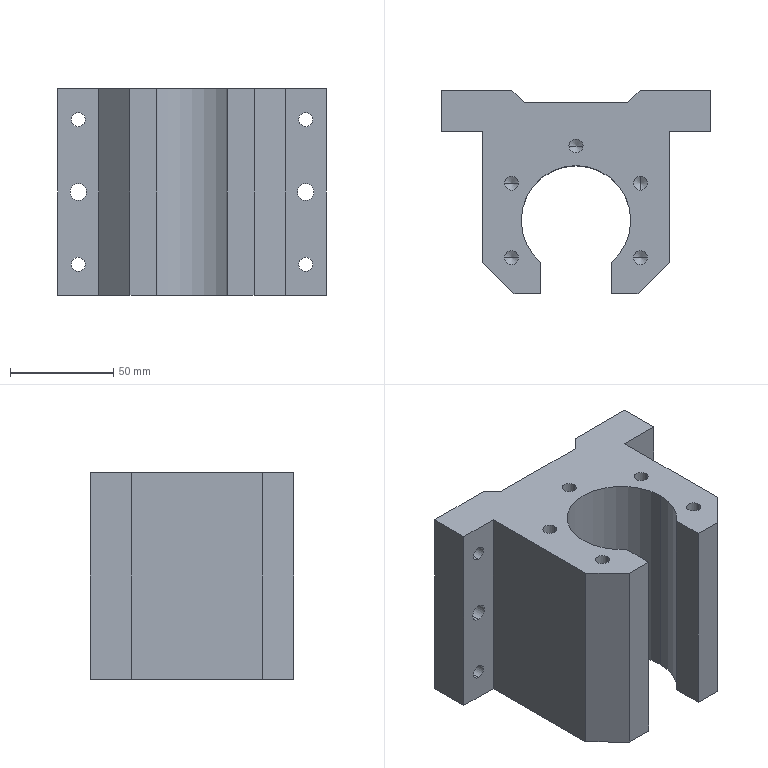Part | STEP file | 40FDD Lead Screw Nut Seat | 1 solid | 54 faces | box 130 x 98.329 x 100 mm | volume 642509 mm3 | cylinder 25 | plane 19 | cone 10 | commonest cylinder face diameters 6.8 x18 8 x4 53 x3